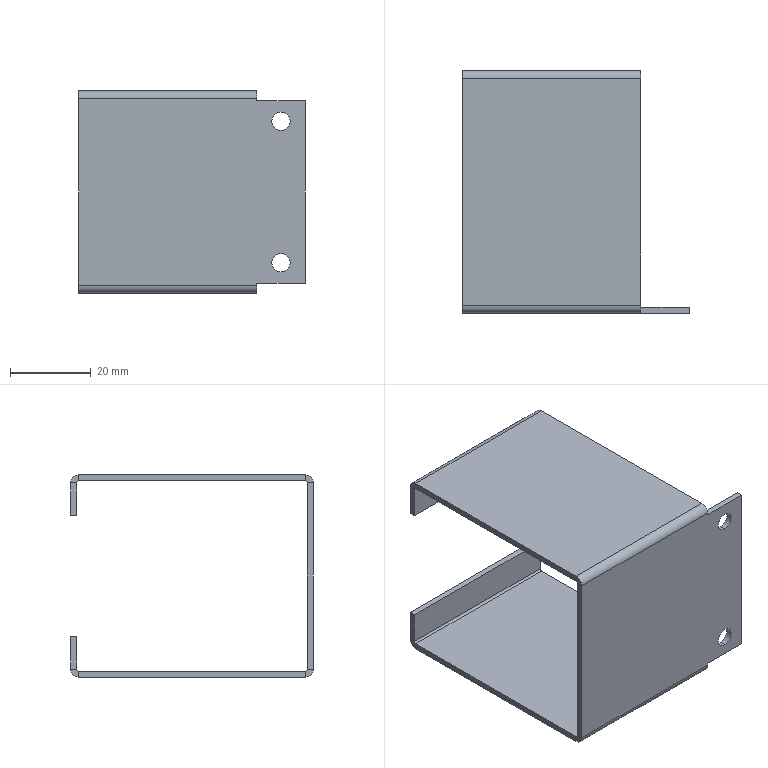Part | STEP file | B1-032 | 1 solid | 46 faces | box 56 x 60 x 50 mm | volume 12765 mm3 | plane 34 | cylinder 12 | commonest cylinder face diameters 1 x4 4 x4 4.5 x4